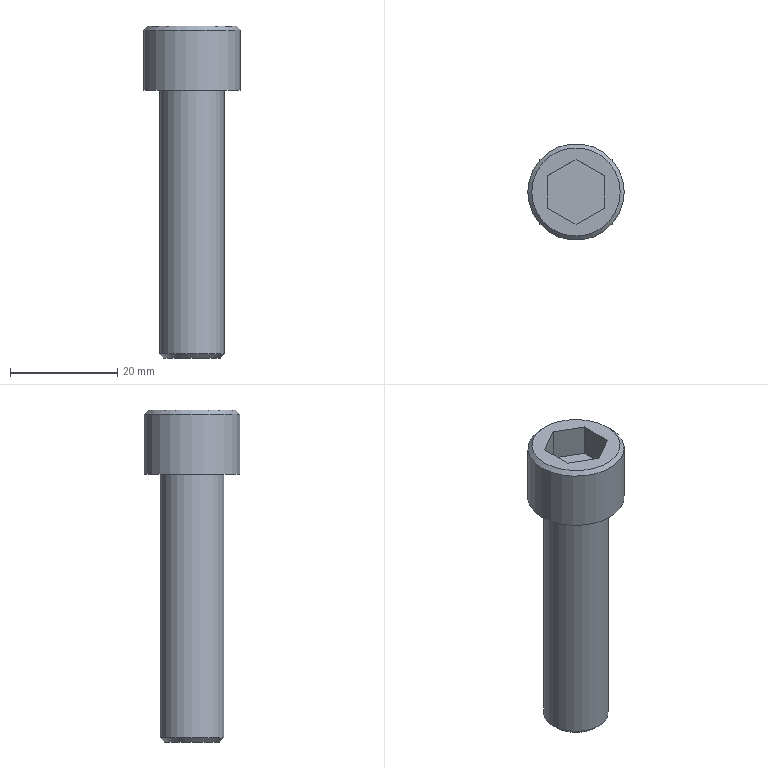Part | STEP file | M12.00-50.00 | 1 solid | 14 faces | box 18 x 18 x 62 mm | volume 8110 mm3 | plane 10 | cylinder 2 | cone 2 | commonest cylinder face diameters 12 x1 18 x1